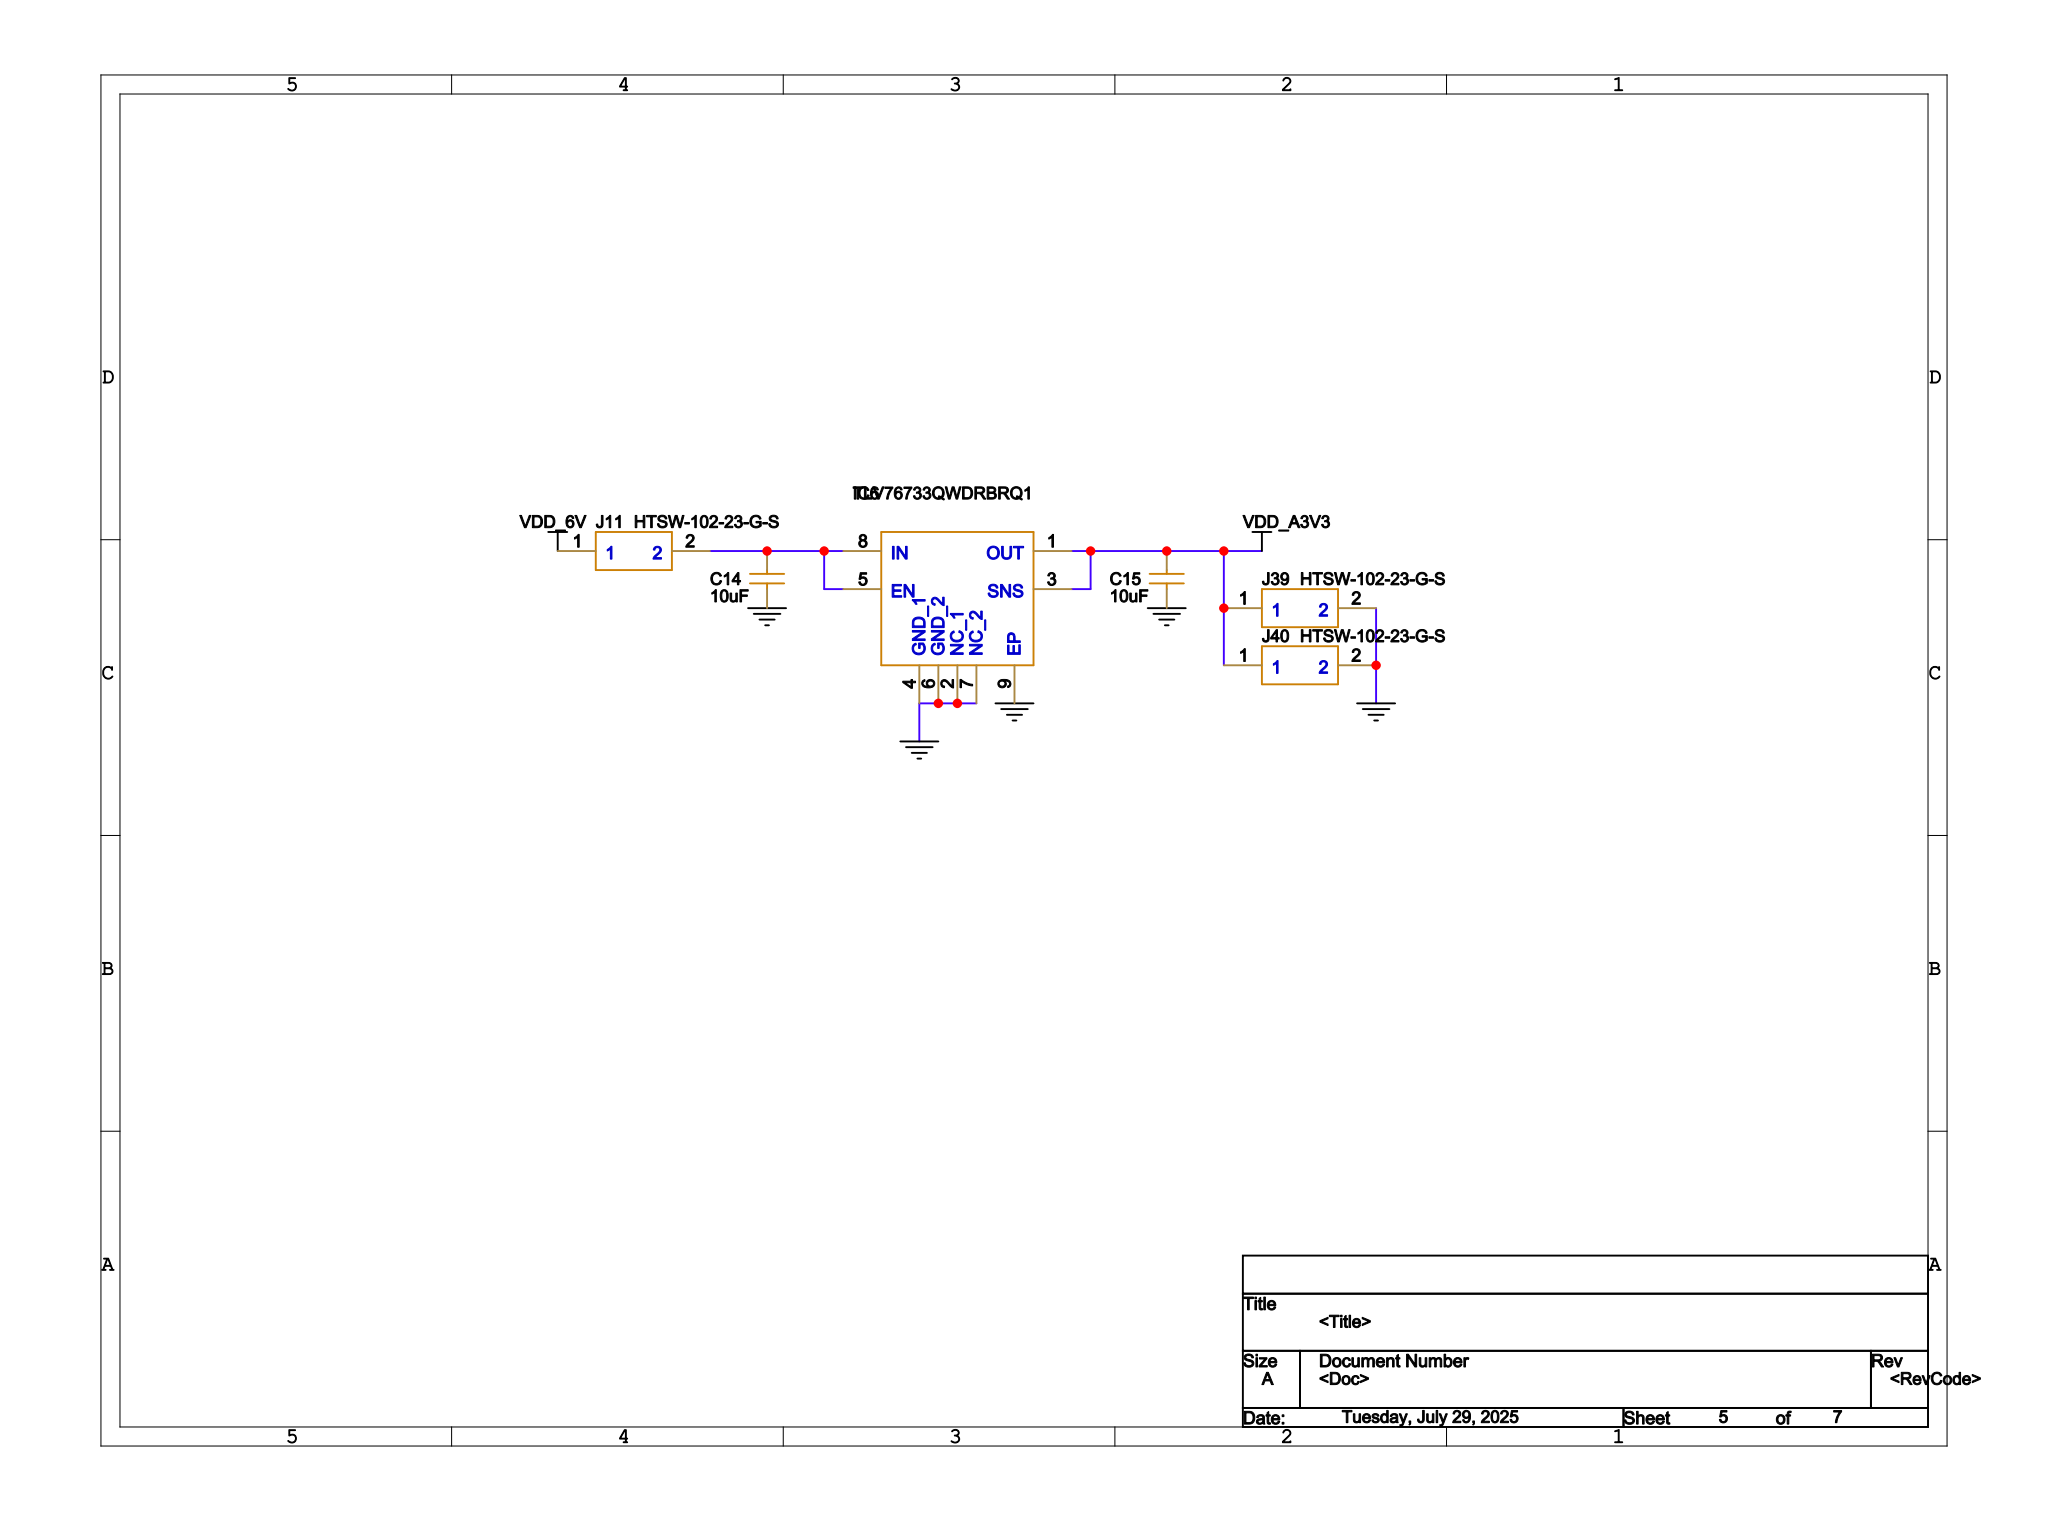Circuit board | Cadence Allegro | 93 parts | 49 nets | one sheet of the schematic
Parts on this sheet (reference | value | footprint):
C14 | 10uF | C1210
C15 | 10uF | C1210
IC6 | TLV76733QWDRBRQ1 | SON65P300X300X100-9N-D
J11 | HTSW-102-23-G-S | HDRV2W64P0X254_1X2_508X248X838P
J39 | HTSW-102-23-G-S | HDRV2W64P0X254_1X2_508X248X838P
J40 | HTSW-102-23-G-S | HDRV2W64P0X254_1X2_508X248X838P
Nets of these parts (net: part-pin ...):
VDD_6V: J11-1
GND: C14-2 C15-2 IC6-2 IC6-4 IC6-6 IC6-7 IC6-9 J39-2 J40-2
N06496: C14-1 IC6-5 IC6-8 J11-2
VDD_A3V3: C15-1 IC6-1 IC6-3 J39-1 J40-1